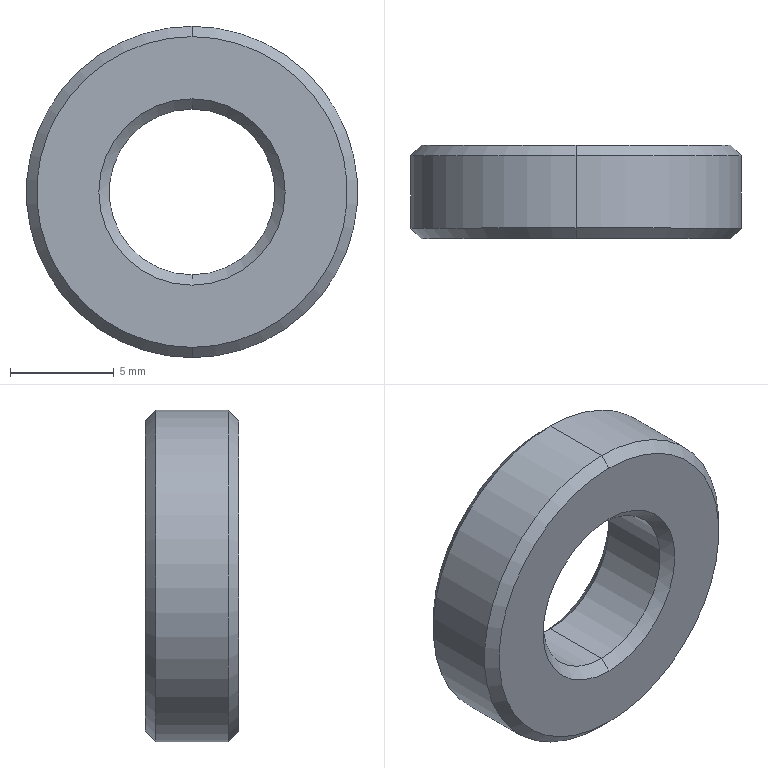Part | SolidWorks | features Chamfer 1, Extrusion 1 | 1 solid | 14 faces | box 16 x 4.5 x 16 mm | volume 659.734 mm3 | cone 8 | cylinder 4 | plane 2 | commonest cylinder face diameters 8 x2 16 x2
STEP:
#1=CARTESIAN_POINT('',(0.,4.5,7.5));
#2=VERTEX_POINT('',#1);
#3=CARTESIAN_POINT('',(0.,4.5,-7.5));
#4=VERTEX_POINT('',#3);
#5=CARTESIAN_POINT('',(0.,4.5,0.));
#6=DIRECTION('',(0.,1.,0.));
#7=DIRECTION('',(0.,0.,1.));
#8=AXIS2_PLACEMENT_3D('',#5,#6,#7);
#9=CIRCLE('',#8,7.5);
#10=EDGE_CURVE('',#2,#4,#9,.T.);
#11=ORIENTED_EDGE('',*,*,#10,.F.);
#12=CARTESIAN_POINT('',(0.,4.,8.));
#13=VERTEX_POINT('',#12);
#14=CARTESIAN_POINT('',(0.,4.5,7.5));
#15=DIRECTION('',(0.,-0.7071,0.7071));
#16=VECTOR('',#15,1000.);
#17=LINE('',#14,#16);
#18=EDGE_CURVE('',#2,#13,#17,.T.);
#19=ORIENTED_EDGE('',*,*,#18,.T.);
#20=CARTESIAN_POINT('',(0.,4.,-8.));
#21=VERTEX_POINT('',#20);
#22=CARTESIAN_POINT('',(0.,4.,0.));
#23=DIRECTION('',(0.,-1.,0.));
#24=DIRECTION('',(0.,0.,1.));
#25=AXIS2_PLACEMENT_3D('',#22,#23,#24);
#26=CIRCLE('',#25,8.);
#27=EDGE_CURVE('',#21,#13,#26,.T.);
#28=ORIENTED_EDGE('',*,*,#27,.F.);
#29=CARTESIAN_POINT('',(0.,4.5,-7.5));
#30=DIRECTION('',(0.,-0.7071,-0.7071));
#31=VECTOR('',#30,1000.);
#32=LINE('',#29,#31);
#33=EDGE_CURVE('',#4,#21,#32,.T.);
#34=ORIENTED_EDGE('',*,*,#33,.F.);
#35=EDGE_LOOP('',(#11,#19,#28,#34));
#36=FACE_OUTER_BOUND('',#35,.T.);
#37=CARTESIAN_POINT('',(0.,4.5,0.));
#38=DIRECTION('',(0.,-1.,0.));
#39=DIRECTION('',(0.,0.,-1.));
#40=AXIS2_PLACEMENT_3D('',#37,#38,#39);
#41=CONICAL_SURFACE('',#40,7.5,0.7854);
#42=ADVANCED_FACE('',(#36),#41,.T.);
#43=CARTESIAN_POINT('',(0.,0.,-7.5));
#44=VERTEX_POINT('',#43);
#45=CARTESIAN_POINT('',(0.,0.,7.5));
#46=VERTEX_POINT('',#45);
#47=CARTESIAN_POINT('',(0.,0.,0.));
#48=DIRECTION('',(0.,-1.,0.));
#49=DIRECTION('',(0.,0.,1.));
#50=AXIS2_PLACEMENT_3D('',#47,#48,#49);
#51=CIRCLE('',#50,7.5);
#52=EDGE_CURVE('',#44,#46,#51,.T.);
#53=ORIENTED_EDGE('',*,*,#52,.F.);
#54=CARTESIAN_POINT('',(0.,0.5,-8.));
#55=VERTEX_POINT('',#54);
#56=CARTESIAN_POINT('',(0.,0.5,-8.));
#57=DIRECTION('',(0.,0.7071,-0.7071));
#58=VECTOR('',#57,1000.);
#59=LINE('',#56,#58);
#60=EDGE_CURVE('',#44,#55,#59,.T.);
#61=ORIENTED_EDGE('',*,*,#60,.T.);
#62=CARTESIAN_POINT('',(0.,0.5,8.));
#63=VERTEX_POINT('',#62);
#64=CARTESIAN_POINT('',(0.,0.5,0.));
#65=DIRECTION('',(0.,1.,0.));
#66=DIRECTION('',(0.,0.,1.));
#67=AXIS2_PLACEMENT_3D('',#64,#65,#66);
#68=CIRCLE('',#67,8.);
#69=EDGE_CURVE('',#63,#55,#68,.T.);
#70=ORIENTED_EDGE('',*,*,#69,.F.);
#71=CARTESIAN_POINT('',(0.,0.5,8.));
#72=DIRECTION('',(0.,0.7071,0.7071));
#73=VECTOR('',#72,1000.);
#74=LINE('',#71,#73);
#75=EDGE_CURVE('',#46,#63,#74,.T.);
#76=ORIENTED_EDGE('',*,*,#75,.F.);
#77=EDGE_LOOP('',(#53,#61,#70,#76));
#78=FACE_OUTER_BOUND('',#77,.T.);
#79=CARTESIAN_POINT('',(0.,0.5,0.));
#80=DIRECTION('',(0.,1.,0.));
#81=DIRECTION('',(0.,0.,1.));
#82=AXIS2_PLACEMENT_3D('',#79,#80,#81);
#83=CONICAL_SURFACE('',#82,8.,0.7854);
#84=ADVANCED_FACE('',(#78),#83,.T.);
#85=CARTESIAN_POINT('',(0.,4.,-4.));
#86=VERTEX_POINT('',#85);
#87=CARTESIAN_POINT('',(0.,4.,4.));
#88=VERTEX_POINT('',#87);
#89=CARTESIAN_POINT('',(0.,4.,0.));
#90=DIRECTION('',(0.,1.,0.));
#91=DIRECTION('',(0.,0.,1.));
#92=AXIS2_PLACEMENT_3D('',#89,#90,#91);
#93=CIRCLE('',#92,4.);
#94=EDGE_CURVE('',#86,#88,#93,.T.);
#95=ORIENTED_EDGE('',*,*,#94,.F.);
#96=CARTESIAN_POINT('',(0.,4.5,-4.5));
#97=VERTEX_POINT('',#96);
#98=CARTESIAN_POINT('',(0.,4.,-4.));
#99=DIRECTION('',(0.,0.7071,-0.7071));
#100=VECTOR('',#99,1000.);
#101=LINE('',#98,#100);
#102=EDGE_CURVE('',#86,#97,#101,.T.);
#103=ORIENTED_EDGE('',*,*,#102,.T.);
#104=CARTESIAN_POINT('',(0.,4.5,4.5));
#105=VERTEX_POINT('',#104);
#106=CARTESIAN_POINT('',(0.,4.5,0.));
#107=DIRECTION('',(0.,-1.,0.));
#108=DIRECTION('',(0.,0.,1.));
#109=AXIS2_PLACEMENT_3D('',#106,#107,#108);
#110=CIRCLE('',#109,4.5);
#111=EDGE_CURVE('',#105,#97,#110,.T.);
#112=ORIENTED_EDGE('',*,*,#111,.F.);
#113=CARTESIAN_POINT('',(0.,4.,4.));
#114=DIRECTION('',(0.,0.7071,0.7071));
#115=VECTOR('',#114,1000.);
#116=LINE('',#113,#115);
#117=EDGE_CURVE('',#88,#105,#116,.T.);
#118=ORIENTED_EDGE('',*,*,#117,.F.);
#119=EDGE_LOOP('',(#95,#103,#112,#118));
#120=FACE_OUTER_BOUND('',#119,.T.);
#121=CARTESIAN_POINT('',(0.,4.,0.));
#122=DIRECTION('',(0.,1.,0.));
#123=DIRECTION('',(0.,0.,1.));
#124=AXIS2_PLACEMENT_3D('',#121,#122,#123);
#125=CONICAL_SURFACE('',#124,4.,0.7854);
#126=ADVANCED_FACE('',(#120),#125,.F.);
#127=CARTESIAN_POINT('',(0.,0.5,4.));
#128=VERTEX_POINT('',#127);
#129=CARTESIAN_POINT('',(0.,0.5,-4.));
#130=VERTEX_POINT('',#129);
#131=CARTESIAN_POINT('',(0.,0.5,0.));
#132=DIRECTION('',(0.,-1.,0.));
#133=DIRECTION('',(0.,0.,1.));
#134=AXIS2_PLACEMENT_3D('',#131,#132,#133);
#135=CIRCLE('',#134,4.);
#136=EDGE_CURVE('',#128,#130,#135,.T.);
#137=ORIENTED_EDGE('',*,*,#136,.F.);
#138=CARTESIAN_POINT('',(0.,0.,4.5));
#139=VERTEX_POINT('',#138);
#140=CARTESIAN_POINT('',(0.,0.,4.5));
#141=DIRECTION('',(0.,-0.7071,0.7071));
#142=VECTOR('',#141,1000.);
#143=LINE('',#140,#142);
#144=EDGE_CURVE('',#128,#139,#143,.T.);
#145=ORIENTED_EDGE('',*,*,#144,.T.);
#146=CARTESIAN_POINT('',(0.,0.,-4.5));
#147=VERTEX_POINT('',#146);
#148=CARTESIAN_POINT('',(0.,0.,0.));
#149=DIRECTION('',(0.,1.,0.));
#150=DIRECTION('',(0.,0.,1.));
#151=AXIS2_PLACEMENT_3D('',#148,#149,#150);
#152=CIRCLE('',#151,4.5);
#153=EDGE_CURVE('',#147,#139,#152,.T.);
#154=ORIENTED_EDGE('',*,*,#153,.F.);
#155=CARTESIAN_POINT('',(0.,0.,-4.5));
#156=DIRECTION('',(0.,-0.7071,-0.7071));
#157=VECTOR('',#156,1000.);
#158=LINE('',#155,#157);
#159=EDGE_CURVE('',#130,#147,#158,.T.);
#160=ORIENTED_EDGE('',*,*,#159,.F.);
#161=EDGE_LOOP('',(#137,#145,#154,#160));
#162=FACE_OUTER_BOUND('',#161,.T.);
#163=CARTESIAN_POINT('',(0.,0.,0.));
#164=DIRECTION('',(0.,-1.,0.));
#165=DIRECTION('',(0.,0.,-1.));
#166=AXIS2_PLACEMENT_3D('',#163,#164,#165);
#167=CONICAL_SURFACE('',#166,4.5,0.7854);
#168=ADVANCED_FACE('',(#162),#167,.F.);
#169=ORIENTED_EDGE('',*,*,#94,.T.);
#170=CARTESIAN_POINT('',(0.,4.5,4.));
#171=DIRECTION('',(0.,-1.,0.));
#172=VECTOR('',#171,1000.);
#173=LINE('',#170,#172);
#174=EDGE_CURVE('',#88,#128,#173,.T.);
#175=ORIENTED_EDGE('',*,*,#174,.T.);
#176=ORIENTED_EDGE('',*,*,#136,.T.);
#177=CARTESIAN_POINT('',(0.,4.5,-4.));
#178=DIRECTION('',(0.,-1.,0.));
#179=VECTOR('',#178,1000.);
#180=LINE('',#177,#179);
#181=EDGE_CURVE('',#86,#130,#180,.T.);
#182=ORIENTED_EDGE('',*,*,#181,.F.);
#183=EDGE_LOOP('',(#169,#175,#176,#182));
#184=FACE_OUTER_BOUND('',#183,.T.);
#185=CARTESIAN_POINT('',(0.,4.5,0.));
#186=DIRECTION('',(0.,-1.,0.));
#187=DIRECTION('',(0.,0.,-1.));
#188=AXIS2_PLACEMENT_3D('',#185,#186,#187);
#189=CYLINDRICAL_SURFACE('',#188,4.);
#190=ADVANCED_FACE('',(#184),#189,.F.);
#191=ORIENTED_EDGE('',*,*,#27,.T.);
#192=CARTESIAN_POINT('',(0.,4.5,8.));
#193=DIRECTION('',(0.,-1.,0.));
#194=VECTOR('',#193,1000.);
#195=LINE('',#192,#194);
#196=EDGE_CURVE('',#13,#63,#195,.T.);
#197=ORIENTED_EDGE('',*,*,#196,.T.);
#198=ORIENTED_EDGE('',*,*,#69,.T.);
#199=CARTESIAN_POINT('',(0.,4.5,-8.));
#200=DIRECTION('',(0.,-1.,0.));
#201=VECTOR('',#200,1000.);
#202=LINE('',#199,#201);
#203=EDGE_CURVE('',#21,#55,#202,.T.);
#204=ORIENTED_EDGE('',*,*,#203,.F.);
#205=EDGE_LOOP('',(#191,#197,#198,#204));
#206=FACE_OUTER_BOUND('',#205,.T.);
#207=CARTESIAN_POINT('',(0.,4.5,0.));
#208=DIRECTION('',(0.,-1.,0.));
#209=DIRECTION('',(0.,0.,-1.));
#210=AXIS2_PLACEMENT_3D('',#207,#208,#209);
#211=CYLINDRICAL_SURFACE('',#210,8.);
#212=ADVANCED_FACE('',(#206),#211,.T.);
#213=ORIENTED_EDGE('',*,*,#111,.T.);
#214=CARTESIAN_POINT('',(0.,4.5,0.));
#215=DIRECTION('',(0.,-1.,0.));
#216=DIRECTION('',(0.,0.,1.));
#217=AXIS2_PLACEMENT_3D('',#214,#215,#216);
#218=CIRCLE('',#217,4.5);
#219=EDGE_CURVE('',#97,#105,#218,.T.);
#220=ORIENTED_EDGE('',*,*,#219,.T.);
#221=EDGE_LOOP('',(#213,#220));
#222=FACE_BOUND('',#221,.T.);
#223=CARTESIAN_POINT('',(0.,4.5,0.));
#224=DIRECTION('',(0.,1.,0.));
#225=DIRECTION('',(0.,0.,1.));
#226=AXIS2_PLACEMENT_3D('',#223,#224,#225);
#227=CIRCLE('',#226,7.5);
#228=EDGE_CURVE('',#4,#2,#227,.T.);
#229=ORIENTED_EDGE('',*,*,#228,.T.);
#230=ORIENTED_EDGE('',*,*,#10,.T.);
#231=EDGE_LOOP('',(#229,#230));
#232=FACE_OUTER_BOUND('',#231,.T.);
#233=CARTESIAN_POINT('',(0.,4.5,0.));
#234=DIRECTION('',(0.,1.,0.));
#235=DIRECTION('',(0.,0.,1.));
#236=AXIS2_PLACEMENT_3D('',#233,#234,#235);
#237=PLANE('',#236);
#238=ADVANCED_FACE('',(#222,#232),#237,.T.);
#239=ORIENTED_EDGE('',*,*,#153,.T.);
#240=CARTESIAN_POINT('',(0.,0.,0.));
#241=DIRECTION('',(0.,1.,0.));
#242=DIRECTION('',(0.,0.,1.));
#243=AXIS2_PLACEMENT_3D('',#240,#241,#242);
#244=CIRCLE('',#243,4.5);
#245=EDGE_CURVE('',#139,#147,#244,.T.);
#246=ORIENTED_EDGE('',*,*,#245,.T.);
#247=EDGE_LOOP('',(#239,#246));
#248=FACE_BOUND('',#247,.T.);
#249=CARTESIAN_POINT('',(0.,0.,0.));
#250=DIRECTION('',(0.,-1.,0.));
#251=DIRECTION('',(0.,0.,1.));
#252=AXIS2_PLACEMENT_3D('',#249,#250,#251);
#253=CIRCLE('',#252,7.5);
#254=EDGE_CURVE('',#46,#44,#253,.T.);
#255=ORIENTED_EDGE('',*,*,#254,.T.);
#256=ORIENTED_EDGE('',*,*,#52,.T.);
#257=EDGE_LOOP('',(#255,#256));
#258=FACE_OUTER_BOUND('',#257,.T.);
#259=CARTESIAN_POINT('',(0.,0.,0.));
#260=DIRECTION('',(0.,1.,0.));
#261=DIRECTION('',(0.,0.,1.));
#262=AXIS2_PLACEMENT_3D('',#259,#260,#261);
#263=PLANE('',#262);
#264=ADVANCED_FACE('',(#248,#258),#263,.F.);
#265=ORIENTED_EDGE('',*,*,#196,.F.);
#266=CARTESIAN_POINT('',(0.,4.,0.));
#267=DIRECTION('',(0.,-1.,0.));
#268=DIRECTION('',(0.,0.,1.));
#269=AXIS2_PLACEMENT_3D('',#266,#267,#268);
#270=CIRCLE('',#269,8.);
#271=EDGE_CURVE('',#13,#21,#270,.T.);
#272=ORIENTED_EDGE('',*,*,#271,.T.);
#273=ORIENTED_EDGE('',*,*,#203,.T.);
#274=CARTESIAN_POINT('',(0.,0.5,0.));
#275=DIRECTION('',(0.,1.,0.));
#276=DIRECTION('',(0.,0.,1.));
#277=AXIS2_PLACEMENT_3D('',#274,#275,#276);
#278=CIRCLE('',#277,8.);
#279=EDGE_CURVE('',#55,#63,#278,.T.);
#280=ORIENTED_EDGE('',*,*,#279,.T.);
#281=EDGE_LOOP('',(#265,#272,#273,#280));
#282=FACE_OUTER_BOUND('',#281,.T.);
#283=CARTESIAN_POINT('',(0.,4.5,0.));
#284=DIRECTION('',(0.,-1.,0.));
#285=DIRECTION('',(0.,0.,-1.));
#286=AXIS2_PLACEMENT_3D('',#283,#284,#285);
#287=CYLINDRICAL_SURFACE('',#286,8.);
#288=ADVANCED_FACE('',(#282),#287,.T.);
#289=ORIENTED_EDGE('',*,*,#174,.F.);
#290=CARTESIAN_POINT('',(0.,4.,0.));
#291=DIRECTION('',(0.,1.,0.));
#292=DIRECTION('',(0.,0.,1.));
#293=AXIS2_PLACEMENT_3D('',#290,#291,#292);
#294=CIRCLE('',#293,4.);
#295=EDGE_CURVE('',#88,#86,#294,.T.);
#296=ORIENTED_EDGE('',*,*,#295,.T.);
#297=ORIENTED_EDGE('',*,*,#181,.T.);
#298=CARTESIAN_POINT('',(0.,0.5,0.));
#299=DIRECTION('',(0.,-1.,0.));
#300=DIRECTION('',(0.,0.,1.));
#301=AXIS2_PLACEMENT_3D('',#298,#299,#300);
#302=CIRCLE('',#301,4.);
#303=EDGE_CURVE('',#130,#128,#302,.T.);
#304=ORIENTED_EDGE('',*,*,#303,.T.);
#305=EDGE_LOOP('',(#289,#296,#297,#304));
#306=FACE_OUTER_BOUND('',#305,.T.);
#307=CARTESIAN_POINT('',(0.,4.5,0.));
#308=DIRECTION('',(0.,-1.,0.));
#309=DIRECTION('',(0.,0.,-1.));
#310=AXIS2_PLACEMENT_3D('',#307,#308,#309);
#311=CYLINDRICAL_SURFACE('',#310,4.);
#312=ADVANCED_FACE('',(#306),#311,.F.);
#313=ORIENTED_EDGE('',*,*,#144,.F.);
#314=ORIENTED_EDGE('',*,*,#303,.F.);
#315=ORIENTED_EDGE('',*,*,#159,.T.);
#316=ORIENTED_EDGE('',*,*,#245,.F.);
#317=EDGE_LOOP('',(#313,#314,#315,#316));
#318=FACE_OUTER_BOUND('',#317,.T.);
#319=CARTESIAN_POINT('',(0.,0.,0.));
#320=DIRECTION('',(0.,-1.,0.));
#321=DIRECTION('',(0.,0.,-1.));
#322=AXIS2_PLACEMENT_3D('',#319,#320,#321);
#323=CONICAL_SURFACE('',#322,4.5,0.7854);
#324=ADVANCED_FACE('',(#318),#323,.F.);
#325=ORIENTED_EDGE('',*,*,#102,.F.);
#326=ORIENTED_EDGE('',*,*,#295,.F.);
#327=ORIENTED_EDGE('',*,*,#117,.T.);
#328=ORIENTED_EDGE('',*,*,#219,.F.);
#329=EDGE_LOOP('',(#325,#326,#327,#328));
#330=FACE_OUTER_BOUND('',#329,.T.);
#331=CARTESIAN_POINT('',(0.,4.,0.));
#332=DIRECTION('',(0.,1.,0.));
#333=DIRECTION('',(0.,0.,1.));
#334=AXIS2_PLACEMENT_3D('',#331,#332,#333);
#335=CONICAL_SURFACE('',#334,4.,0.7854);
#336=ADVANCED_FACE('',(#330),#335,.F.);
#337=ORIENTED_EDGE('',*,*,#60,.F.);
#338=ORIENTED_EDGE('',*,*,#254,.F.);
#339=ORIENTED_EDGE('',*,*,#75,.T.);
#340=ORIENTED_EDGE('',*,*,#279,.F.);
#341=EDGE_LOOP('',(#337,#338,#339,#340));
#342=FACE_OUTER_BOUND('',#341,.T.);
#343=CARTESIAN_POINT('',(0.,0.5,0.));
#344=DIRECTION('',(0.,1.,0.));
#345=DIRECTION('',(0.,0.,1.));
#346=AXIS2_PLACEMENT_3D('',#343,#344,#345);
#347=CONICAL_SURFACE('',#346,8.,0.7854);
#348=ADVANCED_FACE('',(#342),#347,.T.);
#349=ORIENTED_EDGE('',*,*,#18,.F.);
#350=ORIENTED_EDGE('',*,*,#228,.F.);
#351=ORIENTED_EDGE('',*,*,#33,.T.);
#352=ORIENTED_EDGE('',*,*,#271,.F.);
#353=EDGE_LOOP('',(#349,#350,#351,#352));
#354=FACE_OUTER_BOUND('',#353,.T.);
#355=CARTESIAN_POINT('',(0.,4.5,0.));
#356=DIRECTION('',(0.,-1.,0.));
#357=DIRECTION('',(0.,0.,-1.));
#358=AXIS2_PLACEMENT_3D('',#355,#356,#357);
#359=CONICAL_SURFACE('',#358,7.5,0.7854);
#360=ADVANCED_FACE('',(#354),#359,.T.);
#361=CLOSED_SHELL('',(#42,#84,#126,#168,#190,#212,#238,#264,#288,#312,#324,#336,#348,#360));
#362=MANIFOLD_SOLID_BREP('',#361);
#363=CARTESIAN_POINT('',(0.,0.,0.));
#364=DIRECTION('',(0.,0.,1.));
#365=DIRECTION('',(1.,0.,0.));
#366=AXIS2_PLACEMENT_3D('',#363,#364,#365);
#367=(LENGTH_UNIT()NAMED_UNIT(*)SI_UNIT(.MILLI.,.METRE.));
#368=UNCERTAINTY_MEASURE_WITH_UNIT(LENGTH_MEASURE(0.00001),#367,'','');
#369=(NAMED_UNIT(*)PLANE_ANGLE_UNIT()SI_UNIT($,.RADIAN.));
#370=(NAMED_UNIT(*)SI_UNIT($,.STERADIAN.)SOLID_ANGLE_UNIT());
#371=(GEOMETRIC_REPRESENTATION_CONTEXT(3)GLOBAL_UNCERTAINTY_ASSIGNED_CONTEXT((#368))GLOBAL_UNIT_ASSIGNED_CONTEXT((#367,#369,#370))REPRESENTATION_CONTEXT('',''));
#372=ADVANCED_BREP_SHAPE_REPRESENTATION('',(#362,#366),#371);